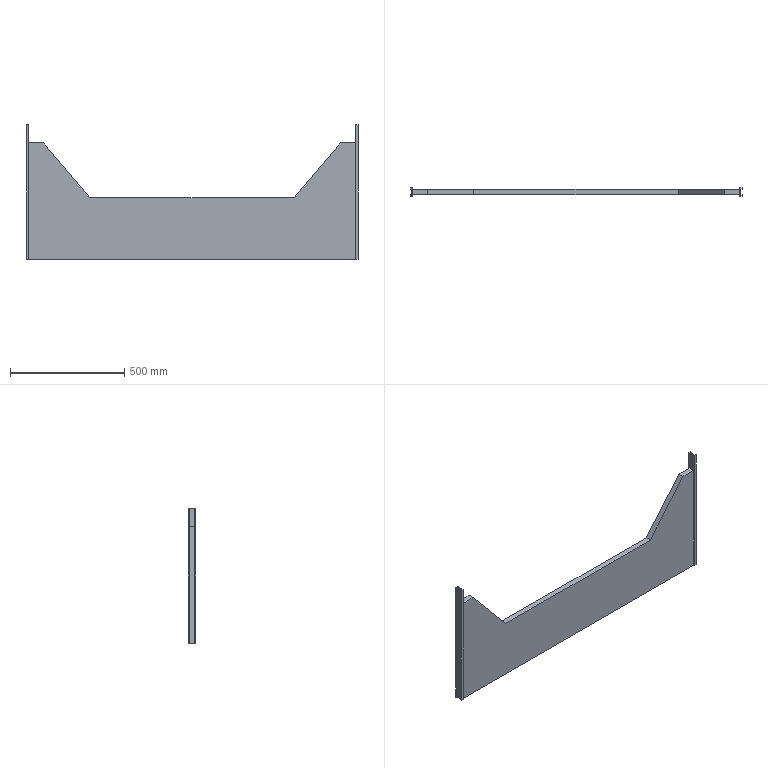Part | SolidWorks | features Extrusion 1, ICE 1 | 1 solid | 26 faces | box 1456 x 35 x 590 mm | volume 11968750 mm3 | plane 26
STEP:
#1=CARTESIAN_POINT('',(0.,-5.,590.));
#2=VERTEX_POINT('',#1);
#3=CARTESIAN_POINT('',(10.,-5.,590.));
#4=VERTEX_POINT('',#3);
#5=CARTESIAN_POINT('',(0.,-5.,590.));
#6=DIRECTION('',(1.,0.,0.));
#7=VECTOR('',#6,1000.);
#8=LINE('',#5,#7);
#9=EDGE_CURVE('',#2,#4,#8,.T.);
#10=ORIENTED_EDGE('',*,*,#9,.T.);
#11=CARTESIAN_POINT('',(10.,30.,590.));
#12=VERTEX_POINT('',#11);
#13=CARTESIAN_POINT('',(10.,25.,590.));
#14=DIRECTION('',(0.,1.,0.));
#15=VECTOR('',#14,1000.);
#16=LINE('',#13,#15);
#17=EDGE_CURVE('',#4,#12,#16,.T.);
#18=ORIENTED_EDGE('',*,*,#17,.T.);
#19=CARTESIAN_POINT('',(0.,30.,590.));
#20=VERTEX_POINT('',#19);
#21=CARTESIAN_POINT('',(10.,30.,590.));
#22=DIRECTION('',(-1.,0.,0.));
#23=VECTOR('',#22,1000.);
#24=LINE('',#21,#23);
#25=EDGE_CURVE('',#12,#20,#24,.T.);
#26=ORIENTED_EDGE('',*,*,#25,.T.);
#27=CARTESIAN_POINT('',(0.,25.,590.));
#28=VERTEX_POINT('',#27);
#29=CARTESIAN_POINT('',(0.,30.,590.));
#30=DIRECTION('',(0.,-1.,0.));
#31=VECTOR('',#30,1000.);
#32=LINE('',#29,#31);
#33=EDGE_CURVE('',#20,#28,#32,.T.);
#34=ORIENTED_EDGE('',*,*,#33,.T.);
#35=CARTESIAN_POINT('',(5.,25.,590.));
#36=VERTEX_POINT('',#35);
#37=CARTESIAN_POINT('',(0.,25.,590.));
#38=DIRECTION('',(1.,0.,0.));
#39=VECTOR('',#38,1000.);
#40=LINE('',#37,#39);
#41=EDGE_CURVE('',#28,#36,#40,.T.);
#42=ORIENTED_EDGE('',*,*,#41,.T.);
#43=CARTESIAN_POINT('',(5.,0.,590.));
#44=VERTEX_POINT('',#43);
#45=CARTESIAN_POINT('',(5.,25.,590.));
#46=DIRECTION('',(0.,-1.,0.));
#47=VECTOR('',#46,1000.);
#48=LINE('',#45,#47);
#49=EDGE_CURVE('',#36,#44,#48,.T.);
#50=ORIENTED_EDGE('',*,*,#49,.T.);
#51=CARTESIAN_POINT('',(0.,0.,590.));
#52=VERTEX_POINT('',#51);
#53=CARTESIAN_POINT('',(5.,0.,590.));
#54=DIRECTION('',(-1.,0.,0.));
#55=VECTOR('',#54,1000.);
#56=LINE('',#53,#55);
#57=EDGE_CURVE('',#44,#52,#56,.T.);
#58=ORIENTED_EDGE('',*,*,#57,.T.);
#59=CARTESIAN_POINT('',(0.,0.,590.));
#60=DIRECTION('',(0.,-1.,0.));
#61=VECTOR('',#60,1000.);
#62=LINE('',#59,#61);
#63=EDGE_CURVE('',#52,#2,#62,.T.);
#64=ORIENTED_EDGE('',*,*,#63,.T.);
#65=EDGE_LOOP('',(#10,#18,#26,#34,#42,#50,#58,#64));
#66=FACE_OUTER_BOUND('',#65,.T.);
#67=CARTESIAN_POINT('',(0.,0.,590.));
#68=DIRECTION('',(0.,0.,-1.));
#69=DIRECTION('',(-1.,0.,0.));
#70=AXIS2_PLACEMENT_3D('',#67,#68,#69);
#71=PLANE('',#70);
#72=ADVANCED_FACE('',(#66),#71,.F.);
#73=CARTESIAN_POINT('',(1456.,30.,0.));
#74=VERTEX_POINT('',#73);
#75=CARTESIAN_POINT('',(1446.,30.,0.));
#76=VERTEX_POINT('',#75);
#77=CARTESIAN_POINT('',(1446.,30.,0.));
#78=DIRECTION('',(-1.,0.,0.));
#79=VECTOR('',#78,1000.);
#80=LINE('',#77,#79);
#81=EDGE_CURVE('',#74,#76,#80,.T.);
#82=ORIENTED_EDGE('',*,*,#81,.T.);
#83=CARTESIAN_POINT('',(1446.,30.,590.));
#84=VERTEX_POINT('',#83);
#85=CARTESIAN_POINT('',(1446.,30.,590.));
#86=DIRECTION('',(0.,0.,-1.));
#87=VECTOR('',#86,1000.);
#88=LINE('',#85,#87);
#89=EDGE_CURVE('',#84,#76,#88,.T.);
#90=ORIENTED_EDGE('',*,*,#89,.F.);
#91=CARTESIAN_POINT('',(1456.,30.,590.));
#92=VERTEX_POINT('',#91);
#93=CARTESIAN_POINT('',(1446.,30.,590.));
#94=DIRECTION('',(-1.,0.,0.));
#95=VECTOR('',#94,1000.);
#96=LINE('',#93,#95);
#97=EDGE_CURVE('',#92,#84,#96,.T.);
#98=ORIENTED_EDGE('',*,*,#97,.F.);
#99=CARTESIAN_POINT('',(1456.,30.,590.));
#100=DIRECTION('',(0.,0.,-1.));
#101=VECTOR('',#100,1000.);
#102=LINE('',#99,#101);
#103=EDGE_CURVE('',#92,#74,#102,.T.);
#104=ORIENTED_EDGE('',*,*,#103,.T.);
#105=EDGE_LOOP('',(#82,#90,#98,#104));
#106=FACE_OUTER_BOUND('',#105,.T.);
#107=CARTESIAN_POINT('',(1446.,30.,590.));
#108=DIRECTION('',(0.,-1.,0.));
#109=DIRECTION('',(0.,0.,-1.));
#110=AXIS2_PLACEMENT_3D('',#107,#108,#109);
#111=PLANE('',#110);
#112=ADVANCED_FACE('',(#106),#111,.F.);
#113=CARTESIAN_POINT('',(10.,25.,510.));
#114=VERTEX_POINT('',#113);
#115=CARTESIAN_POINT('',(10.,25.,0.));
#116=VERTEX_POINT('',#115);
#117=CARTESIAN_POINT('',(10.,25.,590.));
#118=DIRECTION('',(0.,0.,-1.));
#119=VECTOR('',#118,1000.);
#120=LINE('',#117,#119);
#121=EDGE_CURVE('',#114,#116,#120,.T.);
#122=ORIENTED_EDGE('',*,*,#121,.F.);
#123=CARTESIAN_POINT('',(77.5,25.,510.));
#124=VERTEX_POINT('',#123);
#125=CARTESIAN_POINT('',(10.,25.,510.));
#126=DIRECTION('',(-1.,0.,0.));
#127=VECTOR('',#126,1000.);
#128=LINE('',#125,#127);
#129=EDGE_CURVE('',#124,#114,#128,.T.);
#130=ORIENTED_EDGE('',*,*,#129,.F.);
#131=CARTESIAN_POINT('',(280.,25.,270.));
#132=VERTEX_POINT('',#131);
#133=CARTESIAN_POINT('',(77.5,25.,510.));
#134=DIRECTION('',(-0.6449,0.,0.7643));
#135=VECTOR('',#134,1000.);
#136=LINE('',#133,#135);
#137=EDGE_CURVE('',#132,#124,#136,.T.);
#138=ORIENTED_EDGE('',*,*,#137,.F.);
#139=CARTESIAN_POINT('',(1176.,25.,270.));
#140=VERTEX_POINT('',#139);
#141=CARTESIAN_POINT('',(280.,25.,270.));
#142=DIRECTION('',(-1.,0.,0.));
#143=VECTOR('',#142,1000.);
#144=LINE('',#141,#143);
#145=EDGE_CURVE('',#140,#132,#144,.T.);
#146=ORIENTED_EDGE('',*,*,#145,.F.);
#147=CARTESIAN_POINT('',(1378.5,25.,510.));
#148=VERTEX_POINT('',#147);
#149=CARTESIAN_POINT('',(1176.,25.,270.));
#150=DIRECTION('',(-0.6449,0.,-0.7643));
#151=VECTOR('',#150,1000.);
#152=LINE('',#149,#151);
#153=EDGE_CURVE('',#148,#140,#152,.T.);
#154=ORIENTED_EDGE('',*,*,#153,.F.);
#155=CARTESIAN_POINT('',(1446.,25.,510.));
#156=VERTEX_POINT('',#155);
#157=CARTESIAN_POINT('',(1378.5,25.,510.));
#158=DIRECTION('',(-1.,0.,0.));
#159=VECTOR('',#158,1000.);
#160=LINE('',#157,#159);
#161=EDGE_CURVE('',#156,#148,#160,.T.);
#162=ORIENTED_EDGE('',*,*,#161,.F.);
#163=CARTESIAN_POINT('',(1446.,25.,0.));
#164=VERTEX_POINT('',#163);
#165=CARTESIAN_POINT('',(1446.,25.,590.));
#166=DIRECTION('',(0.,0.,-1.));
#167=VECTOR('',#166,1000.);
#168=LINE('',#165,#167);
#169=EDGE_CURVE('',#156,#164,#168,.T.);
#170=ORIENTED_EDGE('',*,*,#169,.T.);
#171=CARTESIAN_POINT('',(10.,25.,0.));
#172=DIRECTION('',(-1.,0.,0.));
#173=VECTOR('',#172,1000.);
#174=LINE('',#171,#173);
#175=EDGE_CURVE('',#164,#116,#174,.T.);
#176=ORIENTED_EDGE('',*,*,#175,.T.);
#177=EDGE_LOOP('',(#122,#130,#138,#146,#154,#162,#170,#176));
#178=FACE_OUTER_BOUND('',#177,.T.);
#179=CARTESIAN_POINT('',(10.,25.,590.));
#180=DIRECTION('',(0.,-1.,0.));
#181=DIRECTION('',(0.,0.,-1.));
#182=AXIS2_PLACEMENT_3D('',#179,#180,#181);
#183=PLANE('',#182);
#184=ADVANCED_FACE('',(#178),#183,.F.);
#185=CARTESIAN_POINT('',(10.,30.,0.));
#186=VERTEX_POINT('',#185);
#187=CARTESIAN_POINT('',(0.,30.,0.));
#188=VERTEX_POINT('',#187);
#189=CARTESIAN_POINT('',(10.,30.,0.));
#190=DIRECTION('',(-1.,0.,0.));
#191=VECTOR('',#190,1000.);
#192=LINE('',#189,#191);
#193=EDGE_CURVE('',#186,#188,#192,.T.);
#194=ORIENTED_EDGE('',*,*,#193,.T.);
#195=CARTESIAN_POINT('',(0.,30.,590.));
#196=DIRECTION('',(0.,0.,-1.));
#197=VECTOR('',#196,1000.);
#198=LINE('',#195,#197);
#199=EDGE_CURVE('',#20,#188,#198,.T.);
#200=ORIENTED_EDGE('',*,*,#199,.F.);
#201=ORIENTED_EDGE('',*,*,#25,.F.);
#202=CARTESIAN_POINT('',(10.,30.,590.));
#203=DIRECTION('',(0.,0.,-1.));
#204=VECTOR('',#203,1000.);
#205=LINE('',#202,#204);
#206=EDGE_CURVE('',#12,#186,#205,.T.);
#207=ORIENTED_EDGE('',*,*,#206,.T.);
#208=EDGE_LOOP('',(#194,#200,#201,#207));
#209=FACE_OUTER_BOUND('',#208,.T.);
#210=CARTESIAN_POINT('',(10.,30.,590.));
#211=DIRECTION('',(0.,-1.,0.));
#212=DIRECTION('',(1.,0.,0.));
#213=AXIS2_PLACEMENT_3D('',#210,#211,#212);
#214=PLANE('',#213);
#215=ADVANCED_FACE('',(#209),#214,.F.);
#216=CARTESIAN_POINT('',(0.,25.,0.));
#217=VERTEX_POINT('',#216);
#218=CARTESIAN_POINT('',(0.,30.,0.));
#219=DIRECTION('',(0.,-1.,0.));
#220=VECTOR('',#219,1000.);
#221=LINE('',#218,#220);
#222=EDGE_CURVE('',#188,#217,#221,.T.);
#223=ORIENTED_EDGE('',*,*,#222,.T.);
#224=CARTESIAN_POINT('',(0.,25.,590.));
#225=DIRECTION('',(0.,0.,-1.));
#226=VECTOR('',#225,1000.);
#227=LINE('',#224,#226);
#228=EDGE_CURVE('',#28,#217,#227,.T.);
#229=ORIENTED_EDGE('',*,*,#228,.F.);
#230=ORIENTED_EDGE('',*,*,#33,.F.);
#231=ORIENTED_EDGE('',*,*,#199,.T.);
#232=EDGE_LOOP('',(#223,#229,#230,#231));
#233=FACE_OUTER_BOUND('',#232,.T.);
#234=CARTESIAN_POINT('',(0.,30.,590.));
#235=DIRECTION('',(1.,0.,0.));
#236=DIRECTION('',(0.,1.,0.));
#237=AXIS2_PLACEMENT_3D('',#234,#235,#236);
#238=PLANE('',#237);
#239=ADVANCED_FACE('',(#233),#238,.F.);
#240=CARTESIAN_POINT('',(5.,25.,0.));
#241=VERTEX_POINT('',#240);
#242=CARTESIAN_POINT('',(0.,25.,0.));
#243=DIRECTION('',(1.,0.,0.));
#244=VECTOR('',#243,1000.);
#245=LINE('',#242,#244);
#246=EDGE_CURVE('',#217,#241,#245,.T.);
#247=ORIENTED_EDGE('',*,*,#246,.T.);
#248=CARTESIAN_POINT('',(5.,25.,590.));
#249=DIRECTION('',(0.,0.,-1.));
#250=VECTOR('',#249,1000.);
#251=LINE('',#248,#250);
#252=EDGE_CURVE('',#36,#241,#251,.T.);
#253=ORIENTED_EDGE('',*,*,#252,.F.);
#254=ORIENTED_EDGE('',*,*,#41,.F.);
#255=ORIENTED_EDGE('',*,*,#228,.T.);
#256=EDGE_LOOP('',(#247,#253,#254,#255));
#257=FACE_OUTER_BOUND('',#256,.T.);
#258=CARTESIAN_POINT('',(0.,25.,590.));
#259=DIRECTION('',(0.,1.,0.));
#260=DIRECTION('',(0.,0.,1.));
#261=AXIS2_PLACEMENT_3D('',#258,#259,#260);
#262=PLANE('',#261);
#263=ADVANCED_FACE('',(#257),#262,.F.);
#264=CARTESIAN_POINT('',(5.,0.,0.));
#265=VERTEX_POINT('',#264);
#266=CARTESIAN_POINT('',(5.,25.,0.));
#267=DIRECTION('',(0.,-1.,0.));
#268=VECTOR('',#267,1000.);
#269=LINE('',#266,#268);
#270=EDGE_CURVE('',#241,#265,#269,.T.);
#271=ORIENTED_EDGE('',*,*,#270,.T.);
#272=CARTESIAN_POINT('',(5.,0.,590.));
#273=DIRECTION('',(0.,0.,-1.));
#274=VECTOR('',#273,1000.);
#275=LINE('',#272,#274);
#276=EDGE_CURVE('',#44,#265,#275,.T.);
#277=ORIENTED_EDGE('',*,*,#276,.F.);
#278=ORIENTED_EDGE('',*,*,#49,.F.);
#279=ORIENTED_EDGE('',*,*,#252,.T.);
#280=EDGE_LOOP('',(#271,#277,#278,#279));
#281=FACE_OUTER_BOUND('',#280,.T.);
#282=CARTESIAN_POINT('',(5.,25.,590.));
#283=DIRECTION('',(1.,0.,0.));
#284=DIRECTION('',(0.,1.,0.));
#285=AXIS2_PLACEMENT_3D('',#282,#283,#284);
#286=PLANE('',#285);
#287=ADVANCED_FACE('',(#281),#286,.F.);
#288=CARTESIAN_POINT('',(0.,0.,0.));
#289=VERTEX_POINT('',#288);
#290=CARTESIAN_POINT('',(5.,0.,0.));
#291=DIRECTION('',(-1.,0.,0.));
#292=VECTOR('',#291,1000.);
#293=LINE('',#290,#292);
#294=EDGE_CURVE('',#265,#289,#293,.T.);
#295=ORIENTED_EDGE('',*,*,#294,.T.);
#296=CARTESIAN_POINT('',(0.,0.,590.));
#297=DIRECTION('',(0.,0.,-1.));
#298=VECTOR('',#297,1000.);
#299=LINE('',#296,#298);
#300=EDGE_CURVE('',#52,#289,#299,.T.);
#301=ORIENTED_EDGE('',*,*,#300,.F.);
#302=ORIENTED_EDGE('',*,*,#57,.F.);
#303=ORIENTED_EDGE('',*,*,#276,.T.);
#304=EDGE_LOOP('',(#295,#301,#302,#303));
#305=FACE_OUTER_BOUND('',#304,.T.);
#306=CARTESIAN_POINT('',(5.,0.,590.));
#307=DIRECTION('',(0.,-1.,0.));
#308=DIRECTION('',(1.,0.,0.));
#309=AXIS2_PLACEMENT_3D('',#306,#307,#308);
#310=PLANE('',#309);
#311=ADVANCED_FACE('',(#305),#310,.F.);
#312=CARTESIAN_POINT('',(0.,-5.,0.));
#313=VERTEX_POINT('',#312);
#314=CARTESIAN_POINT('',(0.,0.,0.));
#315=DIRECTION('',(0.,-1.,0.));
#316=VECTOR('',#315,1000.);
#317=LINE('',#314,#316);
#318=EDGE_CURVE('',#289,#313,#317,.T.);
#319=ORIENTED_EDGE('',*,*,#318,.T.);
#320=CARTESIAN_POINT('',(0.,-5.,590.));
#321=DIRECTION('',(0.,0.,-1.));
#322=VECTOR('',#321,1000.);
#323=LINE('',#320,#322);
#324=EDGE_CURVE('',#2,#313,#323,.T.);
#325=ORIENTED_EDGE('',*,*,#324,.F.);
#326=ORIENTED_EDGE('',*,*,#63,.F.);
#327=ORIENTED_EDGE('',*,*,#300,.T.);
#328=EDGE_LOOP('',(#319,#325,#326,#327));
#329=FACE_OUTER_BOUND('',#328,.T.);
#330=CARTESIAN_POINT('',(0.,0.,590.));
#331=DIRECTION('',(1.,0.,0.));
#332=DIRECTION('',(0.,1.,0.));
#333=AXIS2_PLACEMENT_3D('',#330,#331,#332);
#334=PLANE('',#333);
#335=ADVANCED_FACE('',(#329),#334,.F.);
#336=CARTESIAN_POINT('',(10.,-5.,0.));
#337=VERTEX_POINT('',#336);
#338=CARTESIAN_POINT('',(0.,-5.,0.));
#339=DIRECTION('',(1.,0.,0.));
#340=VECTOR('',#339,1000.);
#341=LINE('',#338,#340);
#342=EDGE_CURVE('',#313,#337,#341,.T.);
#343=ORIENTED_EDGE('',*,*,#342,.T.);
#344=CARTESIAN_POINT('',(10.,-5.,590.));
#345=DIRECTION('',(0.,0.,-1.));
#346=VECTOR('',#345,1000.);
#347=LINE('',#344,#346);
#348=EDGE_CURVE('',#4,#337,#347,.T.);
#349=ORIENTED_EDGE('',*,*,#348,.F.);
#350=ORIENTED_EDGE('',*,*,#9,.F.);
#351=ORIENTED_EDGE('',*,*,#324,.T.);
#352=EDGE_LOOP('',(#343,#349,#350,#351));
#353=FACE_OUTER_BOUND('',#352,.T.);
#354=CARTESIAN_POINT('',(0.,-5.,590.));
#355=DIRECTION('',(0.,1.,0.));
#356=DIRECTION('',(-1.,0.,0.));
#357=AXIS2_PLACEMENT_3D('',#354,#355,#356);
#358=PLANE('',#357);
#359=ADVANCED_FACE('',(#353),#358,.F.);
#360=CARTESIAN_POINT('',(10.,0.,0.));
#361=VERTEX_POINT('',#360);
#362=CARTESIAN_POINT('',(10.,-5.,0.));
#363=DIRECTION('',(0.,1.,0.));
#364=VECTOR('',#363,1000.);
#365=LINE('',#362,#364);
#366=EDGE_CURVE('',#337,#361,#365,.T.);
#367=ORIENTED_EDGE('',*,*,#366,.T.);
#368=CARTESIAN_POINT('',(10.,0.,510.));
#369=VERTEX_POINT('',#368);
#370=CARTESIAN_POINT('',(10.,0.,590.));
#371=DIRECTION('',(0.,0.,-1.));
#372=VECTOR('',#371,1000.);
#373=LINE('',#370,#372);
#374=EDGE_CURVE('',#369,#361,#373,.T.);
#375=ORIENTED_EDGE('',*,*,#374,.F.);
#376=CARTESIAN_POINT('',(10.,-5.001,510.));
#377=DIRECTION('',(0.,1.,0.));
#378=VECTOR('',#377,1000.);
#379=LINE('',#376,#378);
#380=EDGE_CURVE('',#369,#114,#379,.T.);
#381=ORIENTED_EDGE('',*,*,#380,.T.);
#382=ORIENTED_EDGE('',*,*,#121,.T.);
#383=CARTESIAN_POINT('',(10.,25.,0.));
#384=DIRECTION('',(0.,1.,0.));
#385=VECTOR('',#384,1000.);
#386=LINE('',#383,#385);
#387=EDGE_CURVE('',#116,#186,#386,.T.);
#388=ORIENTED_EDGE('',*,*,#387,.T.);
#389=ORIENTED_EDGE('',*,*,#206,.F.);
#390=ORIENTED_EDGE('',*,*,#17,.F.);
#391=ORIENTED_EDGE('',*,*,#348,.T.);
#392=EDGE_LOOP('',(#367,#375,#381,#382,#388,#389,#390,#391));
#393=FACE_OUTER_BOUND('',#392,.T.);
#394=CARTESIAN_POINT('',(10.,-5.,590.));
#395=DIRECTION('',(-1.,0.,0.));
#396=DIRECTION('',(0.,0.,1.));
#397=AXIS2_PLACEMENT_3D('',#394,#395,#396);
#398=PLANE('',#397);
#399=ADVANCED_FACE('',(#393),#398,.F.);
#400=CARTESIAN_POINT('',(77.5,0.,510.));
#401=VERTEX_POINT('',#400);
#402=CARTESIAN_POINT('',(280.,0.,270.));
#403=VERTEX_POINT('',#402);
#404=CARTESIAN_POINT('',(77.5,0.,510.));
#405=DIRECTION('',(0.6449,0.,-0.7643));
#406=VECTOR('',#405,1000.);
#407=LINE('',#404,#406);
#408=EDGE_CURVE('',#401,#403,#407,.T.);
#409=ORIENTED_EDGE('',*,*,#408,.F.);
#410=CARTESIAN_POINT('',(10.,0.,510.));
#411=DIRECTION('',(1.,0.,0.));
#412=VECTOR('',#411,1000.);
#413=LINE('',#410,#412);
#414=EDGE_CURVE('',#369,#401,#413,.T.);
#415=ORIENTED_EDGE('',*,*,#414,.F.);
#416=ORIENTED_EDGE('',*,*,#374,.T.);
#417=CARTESIAN_POINT('',(1446.,0.,0.));
#418=VERTEX_POINT('',#417);
#419=CARTESIAN_POINT('',(10.,0.,0.));
#420=DIRECTION('',(1.,0.,0.));
#421=VECTOR('',#420,1000.);
#422=LINE('',#419,#421);
#423=EDGE_CURVE('',#361,#418,#422,.T.);
#424=ORIENTED_EDGE('',*,*,#423,.T.);
#425=CARTESIAN_POINT('',(1446.,0.,510.));
#426=VERTEX_POINT('',#425);
#427=CARTESIAN_POINT('',(1446.,0.,590.));
#428=DIRECTION('',(0.,0.,-1.));
#429=VECTOR('',#428,1000.);
#430=LINE('',#427,#429);
#431=EDGE_CURVE('',#426,#418,#430,.T.);
#432=ORIENTED_EDGE('',*,*,#431,.F.);
#433=CARTESIAN_POINT('',(1378.5,0.,510.));
#434=VERTEX_POINT('',#433);
#435=CARTESIAN_POINT('',(1378.5,0.,510.));
#436=DIRECTION('',(1.,0.,0.));
#437=VECTOR('',#436,1000.);
#438=LINE('',#435,#437);
#439=EDGE_CURVE('',#434,#426,#438,.T.);
#440=ORIENTED_EDGE('',*,*,#439,.F.);
#441=CARTESIAN_POINT('',(1176.,0.,270.));
#442=VERTEX_POINT('',#441);
#443=CARTESIAN_POINT('',(1176.,0.,270.));
#444=DIRECTION('',(0.6449,0.,0.7643));
#445=VECTOR('',#444,1000.);
#446=LINE('',#443,#445);
#447=EDGE_CURVE('',#442,#434,#446,.T.);
#448=ORIENTED_EDGE('',*,*,#447,.F.);
#449=CARTESIAN_POINT('',(280.,0.,270.));
#450=DIRECTION('',(1.,0.,0.));
#451=VECTOR('',#450,1000.);
#452=LINE('',#449,#451);
#453=EDGE_CURVE('',#403,#442,#452,.T.);
#454=ORIENTED_EDGE('',*,*,#453,.F.);
#455=EDGE_LOOP('',(#409,#415,#416,#424,#432,#440,#448,#454));
#456=FACE_OUTER_BOUND('',#455,.T.);
#457=CARTESIAN_POINT('',(10.,0.,590.));
#458=DIRECTION('',(0.,1.,0.));
#459=DIRECTION('',(0.,0.,1.));
#460=AXIS2_PLACEMENT_3D('',#457,#458,#459);
#461=PLANE('',#460);
#462=ADVANCED_FACE('',(#456),#461,.F.);
#463=CARTESIAN_POINT('',(1446.,-5.,0.));
#464=VERTEX_POINT('',#463);
#465=CARTESIAN_POINT('',(1446.,-5.,0.));
#466=DIRECTION('',(0.,-1.,0.));
#467=VECTOR('',#466,1000.);
#468=LINE('',#465,#467);
#469=EDGE_CURVE('',#418,#464,#468,.T.);
#470=ORIENTED_EDGE('',*,*,#469,.T.);
#471=CARTESIAN_POINT('',(1446.,-5.,590.));
#472=VERTEX_POINT('',#471);
#473=CARTESIAN_POINT('',(1446.,-5.,590.));
#474=DIRECTION('',(0.,0.,-1.));
#475=VECTOR('',#474,1000.);
#476=LINE('',#473,#475);
#477=EDGE_CURVE('',#472,#464,#476,.T.);
#478=ORIENTED_EDGE('',*,*,#477,.F.);
#479=CARTESIAN_POINT('',(1446.,30.,590.));
#480=DIRECTION('',(0.,-1.,0.));
#481=VECTOR('',#480,1000.);
#482=LINE('',#479,#481);
#483=EDGE_CURVE('',#84,#472,#482,.T.);
#484=ORIENTED_EDGE('',*,*,#483,.F.);
#485=ORIENTED_EDGE('',*,*,#89,.T.);
#486=CARTESIAN_POINT('',(1446.,30.,0.));
#487=DIRECTION('',(0.,-1.,0.));
#488=VECTOR('',#487,1000.);
#489=LINE('',#486,#488);
#490=EDGE_CURVE('',#76,#164,#489,.T.);
#491=ORIENTED_EDGE('',*,*,#490,.T.);
#492=ORIENTED_EDGE('',*,*,#169,.F.);
#493=CARTESIAN_POINT('',(1446.,-5.001,510.));
#494=DIRECTION('',(0.,1.,0.));
#495=VECTOR('',#494,1000.);
#496=LINE('',#493,#495);
#497=EDGE_CURVE('',#426,#156,#496,.T.);
#498=ORIENTED_EDGE('',*,*,#497,.F.);
#499=ORIENTED_EDGE('',*,*,#431,.T.);
#500=EDGE_LOOP('',(#470,#478,#484,#485,#491,#492,#498,#499));
#501=FACE_OUTER_BOUND('',#500,.T.);
#502=CARTESIAN_POINT('',(1446.,-5.,590.));
#503=DIRECTION('',(1.,0.,0.));
#504=DIRECTION('',(0.,0.,-1.));
#505=AXIS2_PLACEMENT_3D('',#502,#503,#504);
#506=PLANE('',#505);
#507=ADVANCED_FACE('',(#501),#506,.F.);
#508=CARTESIAN_POINT('',(1456.,-5.,0.));
#509=VERTEX_POINT('',#508);
#510=CARTESIAN_POINT('',(1456.,-5.,0.));
#511=DIRECTION('',(1.,0.,0.));
#512=VECTOR('',#511,1000.);
#513=LINE('',#510,#512);
#514=EDGE_CURVE('',#464,#509,#513,.T.);
#515=ORIENTED_EDGE('',*,*,#514,.T.);
#516=CARTESIAN_POINT('',(1456.,-5.,590.));
#517=VERTEX_POINT('',#516);
#518=CARTESIAN_POINT('',(1456.,-5.,590.));
#519=DIRECTION('',(0.,0.,-1.));
#520=VECTOR('',#519,1000.);
#521=LINE('',#518,#520);
#522=EDGE_CURVE('',#517,#509,#521,.T.);
#523=ORIENTED_EDGE('',*,*,#522,.F.);
#524=CARTESIAN_POINT('',(1456.,-5.,590.));
#525=DIRECTION('',(1.,0.,0.));
#526=VECTOR('',#525,1000.);
#527=LINE('',#524,#526);
#528=EDGE_CURVE('',#472,#517,#527,.T.);
#529=ORIENTED_EDGE('',*,*,#528,.F.);
#530=ORIENTED_EDGE('',*,*,#477,.T.);
#531=EDGE_LOOP('',(#515,#523,#529,#530));
#532=FACE_OUTER_BOUND('',#531,.T.);
#533=CARTESIAN_POINT('',(1456.,-5.,590.));
#534=DIRECTION('',(0.,1.,0.));
#535=DIRECTION('',(-1.,0.,0.));
#536=AXIS2_PLACEMENT_3D('',#533,#534,#535);
#537=PLANE('',#536);
#538=ADVANCED_FACE('',(#532),#537,.F.);
#539=CARTESIAN_POINT('',(1456.,0.,0.));
#540=VERTEX_POINT('',#539);
#541=CARTESIAN_POINT('',(1456.,0.,0.));
#542=DIRECTION('',(0.,1.,0.));
#543=VECTOR('',#542,1000.);
#544=LINE('',#541,#543);
#545=EDGE_CURVE('',#509,#540,#544,.T.);
#546=ORIENTED_EDGE('',*,*,#545,.T.);
#547=CARTESIAN_POINT('',(1456.,0.,590.));
#548=VERTEX_POINT('',#547);
#549=CARTESIAN_POINT('',(1456.,0.,590.));
#550=DIRECTION('',(0.,0.,-1.));
#551=VECTOR('',#550,1000.);
#552=LINE('',#549,#551);
#553=EDGE_CURVE('',#548,#540,#552,.T.);
#554=ORIENTED_EDGE('',*,*,#553,.F.);
#555=CARTESIAN_POINT('',(1456.,0.,590.));
#556=DIRECTION('',(0.,1.,0.));
#557=VECTOR('',#556,1000.);
#558=LINE('',#555,#557);
#559=EDGE_CURVE('',#517,#548,#558,.T.);
#560=ORIENTED_EDGE('',*,*,#559,.F.);
#561=ORIENTED_EDGE('',*,*,#522,.T.);
#562=EDGE_LOOP('',(#546,#554,#560,#561));
#563=FACE_OUTER_BOUND('',#562,.T.);
#564=CARTESIAN_POINT('',(1456.,0.,590.));
#565=DIRECTION('',(-1.,0.,0.));
#566=DIRECTION('',(0.,0.,1.));
#567=AXIS2_PLACEMENT_3D('',#564,#565,#566);
#568=PLANE('',#567);
#569=ADVANCED_FACE('',(#563),#568,.F.);
#570=CARTESIAN_POINT('',(1450.,0.,0.));
#571=VERTEX_POINT('',#570);
#572=CARTESIAN_POINT('',(1450.,0.,0.));
#573=DIRECTION('',(-1.,0.,0.));
#574=VECTOR('',#573,1000.);
#575=LINE('',#572,#574);
#576=EDGE_CURVE('',#540,#571,#575,.T.);
#577=ORIENTED_EDGE('',*,*,#576,.T.);
#578=CARTESIAN_POINT('',(1450.,0.,590.));
#579=VERTEX_POINT('',#578);
#580=CARTESIAN_POINT('',(1450.,0.,590.));
#581=DIRECTION('',(0.,0.,-1.));
#582=VECTOR('',#581,1000.);
#583=LINE('',#580,#582);
#584=EDGE_CURVE('',#579,#571,#583,.T.);
#585=ORIENTED_EDGE('',*,*,#584,.F.);
#586=CARTESIAN_POINT('',(1450.,0.,590.));
#587=DIRECTION('',(-1.,0.,0.));
#588=VECTOR('',#587,1000.);
#589=LINE('',#586,#588);
#590=EDGE_CURVE('',#548,#579,#589,.T.);
#591=ORIENTED_EDGE('',*,*,#590,.F.);
#592=ORIENTED_EDGE('',*,*,#553,.T.);
#593=EDGE_LOOP('',(#577,#585,#591,#592));
#594=FACE_OUTER_BOUND('',#593,.T.);
#595=CARTESIAN_POINT('',(1450.,0.,590.));
#596=DIRECTION('',(0.,-1.,0.));
#597=DIRECTION('',(0.,0.,-1.));
#598=AXIS2_PLACEMENT_3D('',#595,#596,#597);
#599=PLANE('',#598);
#600=ADVANCED_FACE('',(#594),#599,.F.);
#601=CARTESIAN_POINT('',(1450.,25.,0.));
#602=VERTEX_POINT('',#601);
#603=CARTESIAN_POINT('',(1450.,25.,0.));
#604=DIRECTION('',(0.,1.,0.));
#605=VECTOR('',#604,1000.);
#606=LINE('',#603,#605);
#607=EDGE_CURVE('',#571,#602,#606,.T.);
#608=ORIENTED_EDGE('',*,*,#607,.T.);
#609=CARTESIAN_POINT('',(1450.,25.,590.));
#610=VERTEX_POINT('',#609);
#611=CARTESIAN_POINT('',(1450.,25.,590.));
#612=DIRECTION('',(0.,0.,-1.));
#613=VECTOR('',#612,1000.);
#614=LINE('',#611,#613);
#615=EDGE_CURVE('',#610,#602,#614,.T.);
#616=ORIENTED_EDGE('',*,*,#615,.F.);
#617=CARTESIAN_POINT('',(1450.,25.,590.));
#618=DIRECTION('',(0.,1.,0.));
#619=VECTOR('',#618,1000.);
#620=LINE('',#617,#619);
#621=EDGE_CURVE('',#579,#610,#620,.T.);
#622=ORIENTED_EDGE('',*,*,#621,.F.);
#623=ORIENTED_EDGE('',*,*,#584,.T.);
#624=EDGE_LOOP('',(#608,#616,#622,#623));
#625=FACE_OUTER_BOUND('',#624,.T.);
#626=CARTESIAN_POINT('',(1450.,25.,590.));
#627=DIRECTION('',(-1.,0.,0.));
#628=DIRECTION('',(0.,0.,1.));
#629=AXIS2_PLACEMENT_3D('',#626,#627,#628);
#630=PLANE('',#629);
#631=ADVANCED_FACE('',(#625),#630,.F.);
#632=CARTESIAN_POINT('',(1456.,25.,0.));
#633=VERTEX_POINT('',#632);
#634=CARTESIAN_POINT('',(1456.,25.,0.));
#635=DIRECTION('',(1.,0.,0.));
#636=VECTOR('',#635,1000.);
#637=LINE('',#634,#636);
#638=EDGE_CURVE('',#602,#633,#637,.T.);
#639=ORIENTED_EDGE('',*,*,#638,.T.);
#640=CARTESIAN_POINT('',(1456.,25.,590.));
#641=VERTEX_POINT('',#640);
#642=CARTESIAN_POINT('',(1456.,25.,590.));
#643=DIRECTION('',(0.,0.,-1.));
#644=VECTOR('',#643,1000.);
#645=LINE('',#642,#644);
#646=EDGE_CURVE('',#641,#633,#645,.T.);
#647=ORIENTED_EDGE('',*,*,#646,.F.);
#648=CARTESIAN_POINT('',(1456.,25.,590.));
#649=DIRECTION('',(1.,0.,0.));
#650=VECTOR('',#649,1000.);
#651=LINE('',#648,#650);
#652=EDGE_CURVE('',#610,#641,#651,.T.);
#653=ORIENTED_EDGE('',*,*,#652,.F.);
#654=ORIENTED_EDGE('',*,*,#615,.T.);
#655=EDGE_LOOP('',(#639,#647,#653,#654));
#656=FACE_OUTER_BOUND('',#655,.T.);
#657=CARTESIAN_POINT('',(1456.,25.,590.));
#658=DIRECTION('',(0.,1.,0.));
#659=DIRECTION('',(-1.,0.,0.));
#660=AXIS2_PLACEMENT_3D('',#657,#658,#659);
#661=PLANE('',#660);
#662=ADVANCED_FACE('',(#656),#661,.F.);
#663=CARTESIAN_POINT('',(1456.,30.,0.));
#664=DIRECTION('',(0.,1.,0.));
#665=VECTOR('',#664,1000.);
#666=LINE('',#663,#665);
#667=EDGE_CURVE('',#633,#74,#666,.T.);
#668=ORIENTED_EDGE('',*,*,#667,.T.);
#669=ORIENTED_EDGE('',*,*,#103,.F.);
#670=CARTESIAN_POINT('',(1456.,30.,590.));
#671=DIRECTION('',(0.,1.,0.));
#672=VECTOR('',#671,1000.);
#673=LINE('',#670,#672);
#674=EDGE_CURVE('',#641,#92,#673,.T.);
#675=ORIENTED_EDGE('',*,*,#674,.F.);
#676=ORIENTED_EDGE('',*,*,#646,.T.);
#677=EDGE_LOOP('',(#668,#669,#675,#676));
#678=FACE_OUTER_BOUND('',#677,.T.);
#679=CARTESIAN_POINT('',(1456.,30.,590.));
#680=DIRECTION('',(-1.,0.,0.));
#681=DIRECTION('',(0.,0.,1.));
#682=AXIS2_PLACEMENT_3D('',#679,#680,#681);
#683=PLANE('',#682);
#684=ADVANCED_FACE('',(#678),#683,.F.);
#685=ORIENTED_EDGE('',*,*,#483,.T.);
#686=ORIENTED_EDGE('',*,*,#528,.T.);
#687=ORIENTED_EDGE('',*,*,#559,.T.);
#688=ORIENTED_EDGE('',*,*,#590,.T.);
#689=ORIENTED_EDGE('',*,*,#621,.T.);
#690=ORIENTED_EDGE('',*,*,#652,.T.);
#691=ORIENTED_EDGE('',*,*,#674,.T.);
#692=ORIENTED_EDGE('',*,*,#97,.T.);
#693=EDGE_LOOP('',(#685,#686,#687,#688,#689,#690,#691,#692));
#694=FACE_OUTER_BOUND('',#693,.T.);
#695=CARTESIAN_POINT('',(0.,0.,590.));
#696=DIRECTION('',(0.,0.,-1.));
#697=DIRECTION('',(-1.,0.,0.));
#698=AXIS2_PLACEMENT_3D('',#695,#696,#697);
#699=PLANE('',#698);
#700=ADVANCED_FACE('',(#694),#699,.F.);
#701=ORIENTED_EDGE('',*,*,#81,.F.);
#702=ORIENTED_EDGE('',*,*,#667,.F.);
#703=ORIENTED_EDGE('',*,*,#638,.F.);
#704=ORIENTED_EDGE('',*,*,#607,.F.);
#705=ORIENTED_EDGE('',*,*,#576,.F.);
#706=ORIENTED_EDGE('',*,*,#545,.F.);
#707=ORIENTED_EDGE('',*,*,#514,.F.);
#708=ORIENTED_EDGE('',*,*,#469,.F.);
#709=ORIENTED_EDGE('',*,*,#423,.F.);
#710=ORIENTED_EDGE('',*,*,#366,.F.);
#711=ORIENTED_EDGE('',*,*,#342,.F.);
#712=ORIENTED_EDGE('',*,*,#318,.F.);
#713=ORIENTED_EDGE('',*,*,#294,.F.);
#714=ORIENTED_EDGE('',*,*,#270,.F.);
#715=ORIENTED_EDGE('',*,*,#246,.F.);
#716=ORIENTED_EDGE('',*,*,#222,.F.);
#717=ORIENTED_EDGE('',*,*,#193,.F.);
#718=ORIENTED_EDGE('',*,*,#387,.F.);
#719=ORIENTED_EDGE('',*,*,#175,.F.);
#720=ORIENTED_EDGE('',*,*,#490,.F.);
#721=EDGE_LOOP('',(#701,#702,#703,#704,#705,#706,#707,#708,#709,#710,#711,#712,#713,#714,#715,#716,#717,#718,#719,#720));
#722=FACE_OUTER_BOUND('',#721,.T.);
#723=CARTESIAN_POINT('',(0.,0.,0.));
#724=DIRECTION('',(0.,0.,-1.));
#725=DIRECTION('',(-1.,0.,0.));
#726=AXIS2_PLACEMENT_3D('',#723,#724,#725);
#727=PLANE('',#726);
#728=ADVANCED_FACE('',(#722),#727,.T.);
#729=ORIENTED_EDGE('',*,*,#414,.T.);
#730=CARTESIAN_POINT('',(77.5,-5.001,510.));
#731=DIRECTION('',(0.,1.,0.));
#732=VECTOR('',#731,1000.);
#733=LINE('',#730,#732);
#734=EDGE_CURVE('',#401,#124,#733,.T.);
#735=ORIENTED_EDGE('',*,*,#734,.T.);
#736=ORIENTED_EDGE('',*,*,#129,.T.);
#737=ORIENTED_EDGE('',*,*,#380,.F.);
#738=EDGE_LOOP('',(#729,#735,#736,#737));
#739=FACE_OUTER_BOUND('',#738,.T.);
#740=CARTESIAN_POINT('',(10.,-5.001,510.));
#741=DIRECTION('',(0.,0.,-1.));
#742=DIRECTION('',(-1.,0.,0.));
#743=AXIS2_PLACEMENT_3D('',#740,#741,#742);
#744=PLANE('',#743);
#745=ADVANCED_FACE('',(#739),#744,.F.);
#746=ORIENTED_EDGE('',*,*,#408,.T.);
#747=CARTESIAN_POINT('',(280.,-5.001,270.));
#748=DIRECTION('',(0.,1.,0.));
#749=VECTOR('',#748,1000.);
#750=LINE('',#747,#749);
#751=EDGE_CURVE('',#403,#132,#750,.T.);
#752=ORIENTED_EDGE('',*,*,#751,.T.);
#753=ORIENTED_EDGE('',*,*,#137,.T.);
#754=ORIENTED_EDGE('',*,*,#734,.F.);
#755=EDGE_LOOP('',(#746,#752,#753,#754));
#756=FACE_OUTER_BOUND('',#755,.T.);
#757=CARTESIAN_POINT('',(77.5,-5.001,510.));
#758=DIRECTION('',(-0.7643,0.,-0.6449));
#759=DIRECTION('',(-0.6449,0.,0.7643));
#760=AXIS2_PLACEMENT_3D('',#757,#758,#759);
#761=PLANE('',#760);
#762=ADVANCED_FACE('',(#756),#761,.F.);
#763=ORIENTED_EDGE('',*,*,#453,.T.);
#764=CARTESIAN_POINT('',(1176.,-5.001,270.));
#765=DIRECTION('',(0.,1.,0.));
#766=VECTOR('',#765,1000.);
#767=LINE('',#764,#766);
#768=EDGE_CURVE('',#442,#140,#767,.T.);
#769=ORIENTED_EDGE('',*,*,#768,.T.);
#770=ORIENTED_EDGE('',*,*,#145,.T.);
#771=ORIENTED_EDGE('',*,*,#751,.F.);
#772=EDGE_LOOP('',(#763,#769,#770,#771));
#773=FACE_OUTER_BOUND('',#772,.T.);
#774=CARTESIAN_POINT('',(280.,-5.001,270.));
#775=DIRECTION('',(0.,0.,-1.));
#776=DIRECTION('',(-1.,0.,0.));
#777=AXIS2_PLACEMENT_3D('',#774,#775,#776);
#778=PLANE('',#777);
#779=ADVANCED_FACE('',(#773),#778,.F.);
#780=ORIENTED_EDGE('',*,*,#447,.T.);
#781=CARTESIAN_POINT('',(1378.5,-5.001,510.));
#782=DIRECTION('',(0.,1.,0.));
#783=VECTOR('',#782,1000.);
#784=LINE('',#781,#783);
#785=EDGE_CURVE('',#434,#148,#784,.T.);
#786=ORIENTED_EDGE('',*,*,#785,.T.);
#787=ORIENTED_EDGE('',*,*,#153,.T.);
#788=ORIENTED_EDGE('',*,*,#768,.F.);
#789=EDGE_LOOP('',(#780,#786,#787,#788));
#790=FACE_OUTER_BOUND('',#789,.T.);
#791=CARTESIAN_POINT('',(1176.,-5.001,270.));
#792=DIRECTION('',(0.7643,0.,-0.6449));
#793=DIRECTION('',(-0.6449,0.,-0.7643));
#794=AXIS2_PLACEMENT_3D('',#791,#792,#793);
#795=PLANE('',#794);
#796=ADVANCED_FACE('',(#790),#795,.F.);
#797=ORIENTED_EDGE('',*,*,#439,.T.);
#798=ORIENTED_EDGE('',*,*,#497,.T.);
#799=ORIENTED_EDGE('',*,*,#161,.T.);
#800=ORIENTED_EDGE('',*,*,#785,.F.);
#801=EDGE_LOOP('',(#797,#798,#799,#800));
#802=FACE_OUTER_BOUND('',#801,.T.);
#803=CARTESIAN_POINT('',(1378.5,-5.001,510.));
#804=DIRECTION('',(0.,0.,-1.));
#805=DIRECTION('',(-1.,0.,0.));
#806=AXIS2_PLACEMENT_3D('',#803,#804,#805);
#807=PLANE('',#806);
#808=ADVANCED_FACE('',(#802),#807,.F.);
#809=CLOSED_SHELL('',(#72,#112,#184,#215,#239,#263,#287,#311,#335,#359,#399,#462,#507,#538,#569,#600,#631,#662,#684,#700,#728,#745,#762,#779,#796,#808));
#810=MANIFOLD_SOLID_BREP('',#809);
#811=CARTESIAN_POINT('',(0.,0.,0.));
#812=DIRECTION('',(0.,0.,1.));
#813=DIRECTION('',(1.,0.,0.));
#814=AXIS2_PLACEMENT_3D('',#811,#812,#813);
#815=(LENGTH_UNIT()NAMED_UNIT(*)SI_UNIT(.MILLI.,.METRE.));
#816=UNCERTAINTY_MEASURE_WITH_UNIT(LENGTH_MEASURE(0.00001),#815,'','');
#817=(NAMED_UNIT(*)PLANE_ANGLE_UNIT()SI_UNIT($,.RADIAN.));
#818=(NAMED_UNIT(*)SI_UNIT($,.STERADIAN.)SOLID_ANGLE_UNIT());
#819=(GEOMETRIC_REPRESENTATION_CONTEXT(3)GLOBAL_UNCERTAINTY_ASSIGNED_CONTEXT((#816))GLOBAL_UNIT_ASSIGNED_CONTEXT((#815,#817,#818))REPRESENTATION_CONTEXT('',''));
#820=ADVANCED_BREP_SHAPE_REPRESENTATION('',(#810,#814),#819);